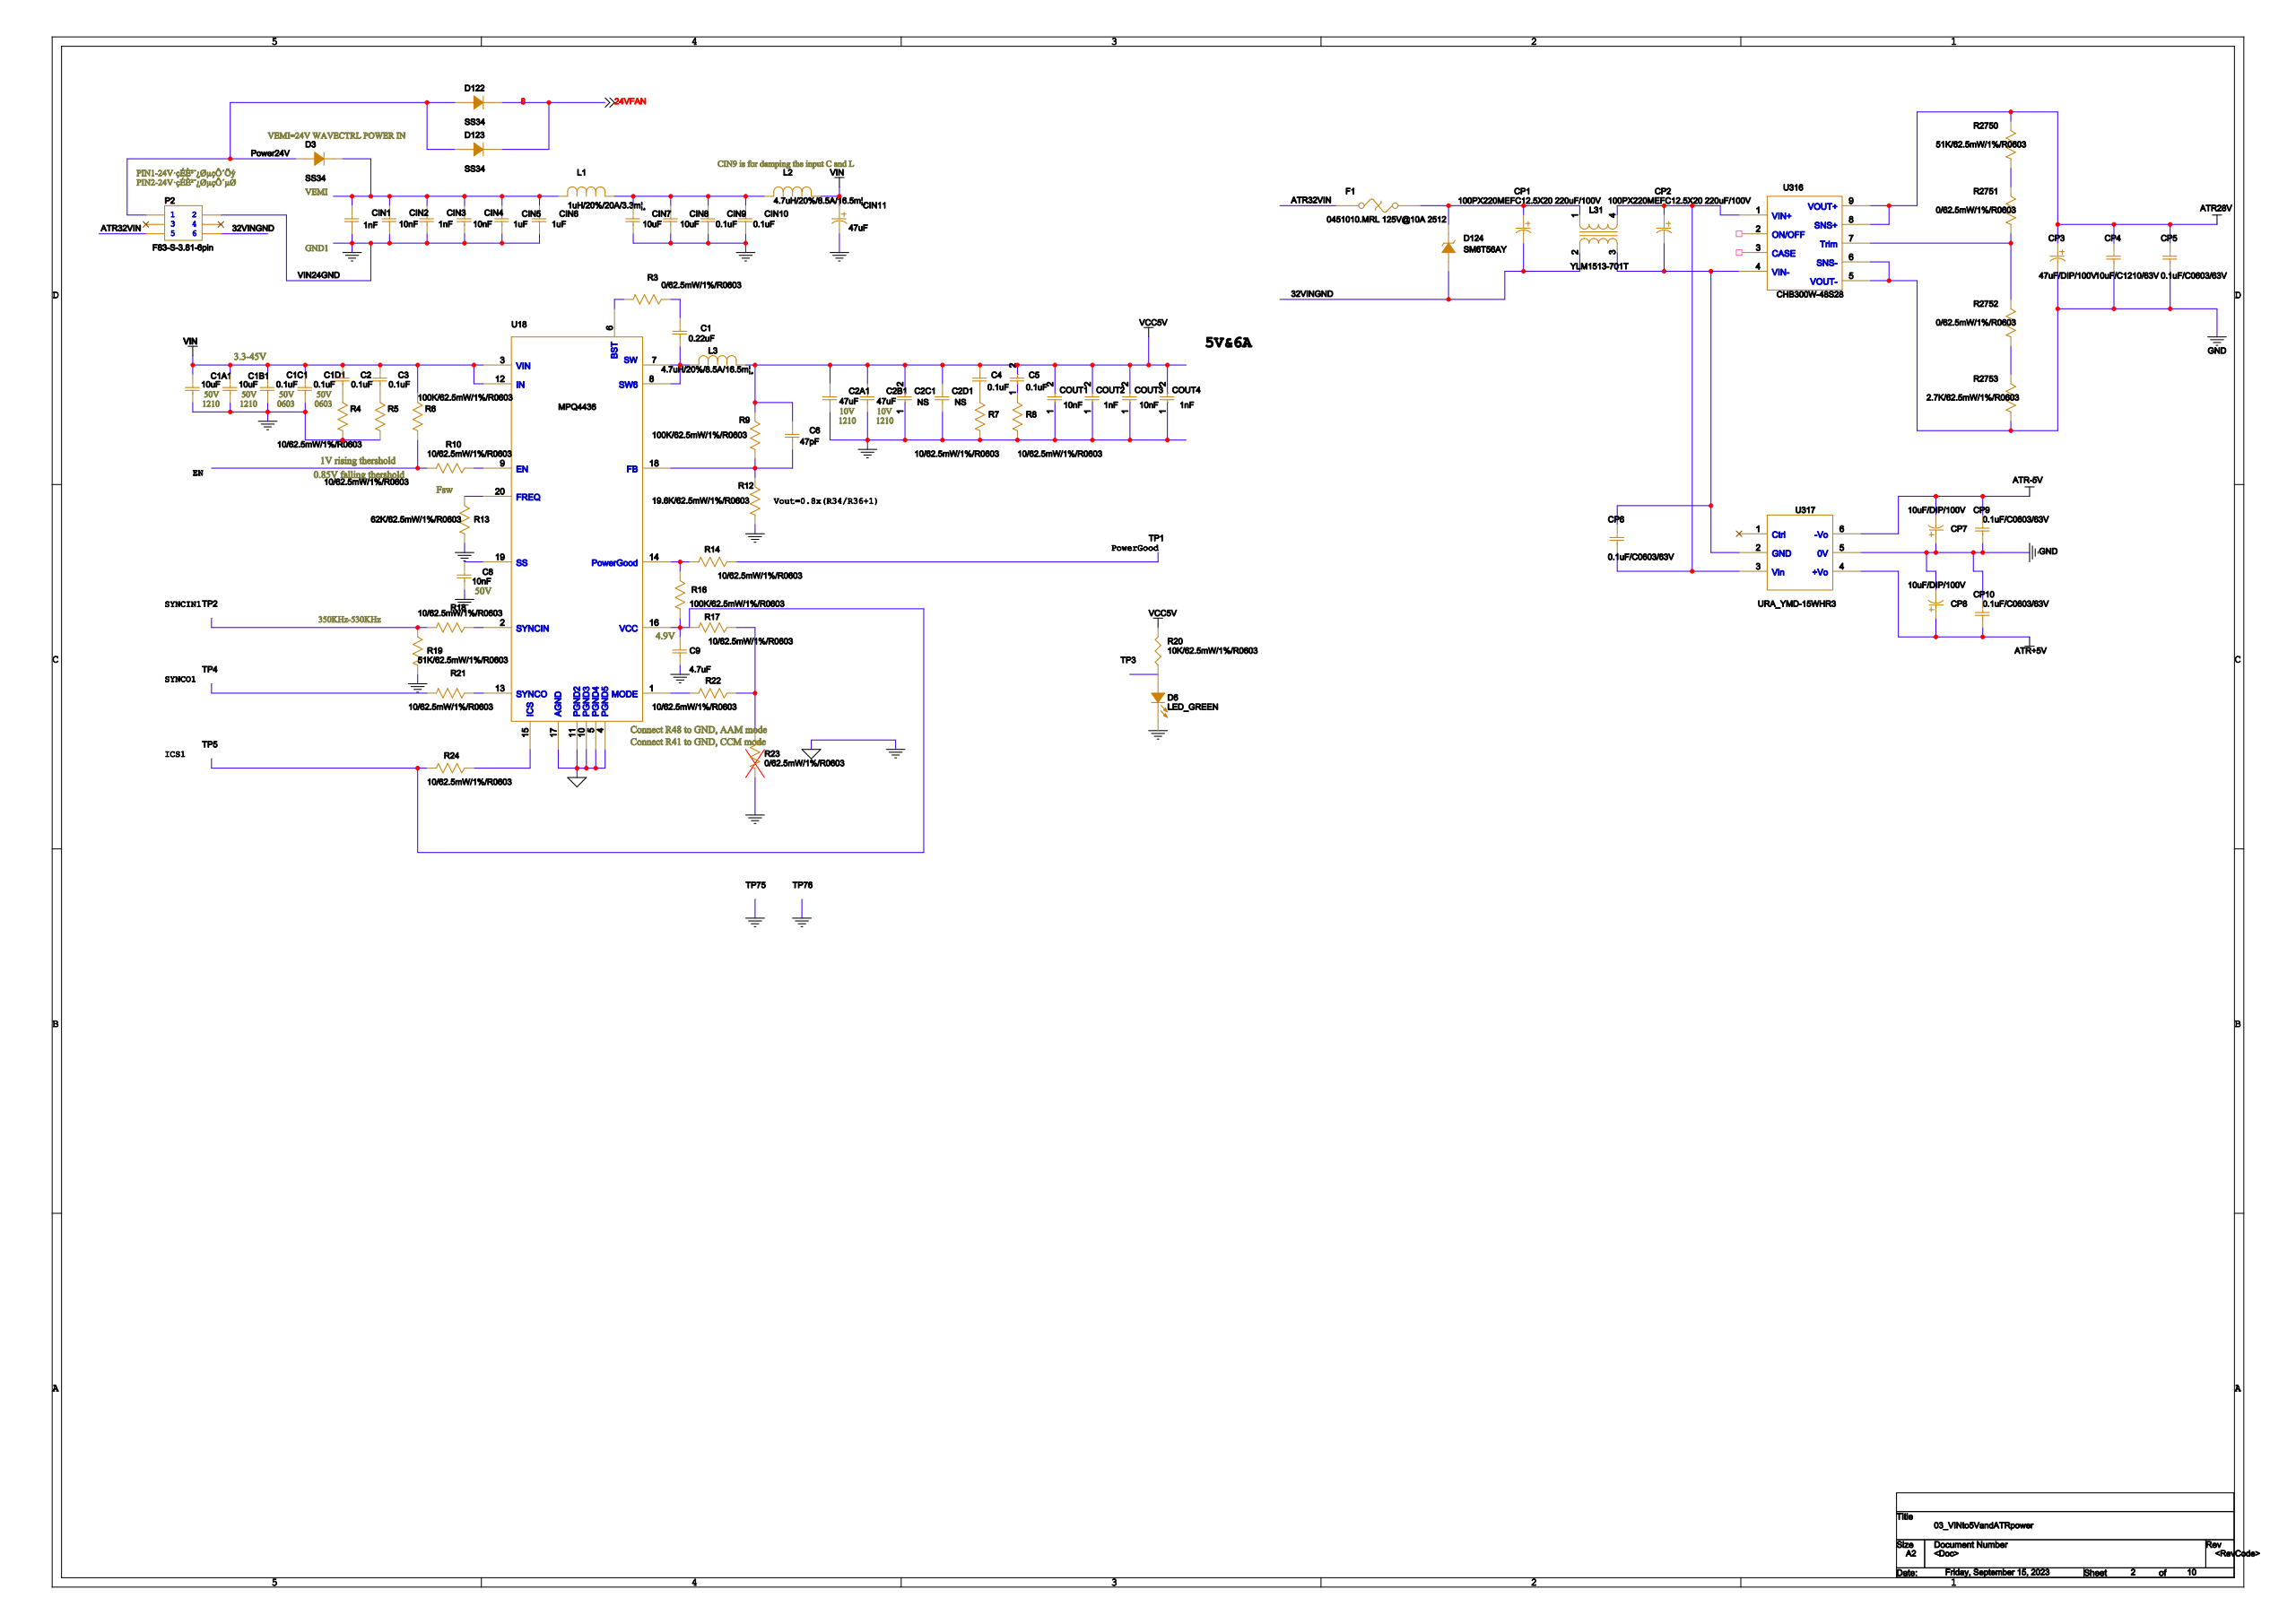Circuit board | Cadence Allegro | 634 parts | 645 nets | one sheet of the schematic
Parts on this sheet (reference | value | footprint):
C1 | CAP/0603 | 0603C
C1A1 | CAP/1210 | 1210
C1B1 | CAP/1210 | 1210
C1C1 | CAP/0603 | 0603C
C1D1 | CAP/0603 | 0603C
C2 | CAP/0603 | 0603C
C2A1 | CAP/1210 | 1210
C2B1 | CAP/1210 | 1210
C2C1 | CAP/0603 | 0603C
C2D1 | CAP/0603 | 0603C
C3 | CAP/0603 | 0603C
C4 | CAP/0603 | 0603C
C5 | CAP/0603 | 0603C
C6 | CAP/0603 | 0603C
C8 | CAP/0603 | 0603C
C9 | CAP/0603 | 0603C
CIN1 | CAP/0603 | 0603C
CIN2 | CAP/0603 | 0603C
CIN3 | CAP/0603 | 0603C
CIN4 | CAP/0603 | 0603C
CIN5 | CAP/0603 | 0805C
CIN6 | CAP/0603 | 0805C
CIN7 | CAP/0603 | 1206
CIN8 | CAP/0603 | 1206
CIN9 | CAP/0603 | 0603C
CIN10 | CAP/0603 | 0603C
CIN11 | CAP/ELECT/DIP/OD5.3P2.0 | AP-SMD_BD6_3-L6_6-W6_6-LS7_21
COUT1 | CAP/0603 | 0603C
COUT2 | CAP/0603 | 0603C
COUT3 | CAP/0603 | 0603C
COUT4 | CAP/0603 | 0603C
CP1 | CAP/ELECT/DIP/OD5.3P2.0 | AP-SMD_BD12_5-L20
CP2 | CAP/ELECT/DIP/OD5.3P2.0 | AP-SMD_BD12_5-L20
CP3 | CAP/ELECT/DIP/OD5.3P2.0 | AP-SMD_BD6_3-L6_6-W6_6-LS7_21
CP4 | CAP/1210 | 1210
CP5 | CAP/0603 | 0603C
CP6 | CAP/0603 | 0603C
CP7 | CAP/ELECT/DIP/OD5.3P2.0 | AP-SMD_BD6_3-L6_6-W6_6-LS7_21
CP8 | CAP/ELECT/DIP/OD5.3P2.0 | AP-SMD_BD6_3-L6_6-W6_6-LS7_21
CP9 | CAP/0603 | 0603C
CP10 | CAP/0603 | 0603C
D3 | SS34 | DO-214AC
D6 | LED_GREEN | LED0805
D122 | SS34 | DO-214AC
D123 | SS34 | DO-214AC
D124 | SM6T56AY | DO-214AA
F1 | 0451010.MRL 125V@10A 2512 | 2512
L1 | CKST1004-1uH/M-B | SMD_10X11
L2 | CKST1004-4.7uH/M | SMD_10X11
L3 | CKST1004-4.7uH/M | SMD_10X11
L31 | YLM1513-701T | SMD_7X6MM
P2 | F83-S-3.81-6pin | F83-S-3_81-6PIN
R3 | 0/62.5mW/1%/R0603 | 0603R
R4 | 10/62.5mW/1%/R0603 | 0603R
R5 | 10/62.5mW/1%/R0603 | 0603R
R6 | 100K/62.5mW/1%/R0603 | 0603R
R7 | 10/62.5mW/1%/R0603 | 0603R
R8 | 10/62.5mW/1%/R0603 | 0603R
R9 | 100K/62.5mW/1%/R0603 | 0603R
R10 | 10/62.5mW/1%/R0603 | 0603R
R12 | 19.6K/62.5mW/1%/R0603 | 0603R
R13 | 62K/62.5mW/1%/R0603 | 0603R
R14 | 10/62.5mW/1%/R0603 | 0603R
R16 | 100K/62.5mW/1%/R0603 | 0603R
R17 | 10/62.5mW/1%/R0603 | 0603R
R18 | 10/62.5mW/1%/R0603 | 0603R
R19 | 51K/62.5mW/1%/R0603 | 0603R
R20 | 10K/62.5mW/1%/R0603 | 0603R
R21 | 10/62.5mW/1%/R0603 | 0603R
R22 | 10/62.5mW/1%/R0603 | 0603R
R23 | 0/62.5mW/1%/R0603 | 0603R
R24 | 10/62.5mW/1%/R0603 | 0603R
R2751 | 0/62.5mW/1%/R0603 | 0603R
R2752 | 0/62.5mW/1%/R0603 | 0603R
R2753 | 2.7K/62.5mW/1%/R0603 | 0603R
TP1 | TEST POINT A | TEST_12MM
TP2 | TEST POINT A | TEST_12MM
TP3 | TEST POINT A | TEST_12MM
TP4 | TEST POINT A | TEST_12MM
TP5 | TEST POINT A | TEST_12MM
TP75 | TEST POINT A | TEST_1MM
TP76 | TEST POINT A | TEST_1MM
U18 | MPQ4436 | QFN-4X4_MPQ4436-AEC1_MNP
U316 | CHB300W-48S28 | CHB300W-48S28
U317 | URA_YMD-15WHR3 | URA_YMD-15WHR3
Nets of these parts (net: part-pin ...):
ATR+5V: CP8-1 CP10-2 U317-4
AGND: C1A1-2 C1B1-2 C1C1-2 C1D1-2 C2A1-2 C2B1-2 C2C1-1 C2D1-1 C8-2 C9-2 CIN1-2 CIN2-2 CIN3-2 CIN4-2 CIN5-2 CIN6-2 CIN7-2 CIN8-2 CIN9-2 CIN10-2 CIN11-2 COUT1-1 COUT2-1 COUT3-1 COUT4-1 CP3-2 CP4-2 CP5-2 CP7-1 CP8-2 CP9-2 CP10-1 D6-2 P2-2 R4-2 R5-2 R7-2 R8-2 R12-1 R13-2 R19-1 R23-2 R2753-1 TP75-1 TP76-1 U18-4 U18-5 U18-10 U18-11 U18-17 U316-5 U316-6 U317-5
ATR28V: CP3-1 CP4-1 CP5-1 U316-8 U316-9
N24674723: CP1-1 D124-1 F1-2 L31-1
32VINGND: CP1-2 D124-2 L31-2 P2-6
N24674699: CP2-1 CP6-2 L31-4 U316-1 U317-3
N24674686: CP2-2 CP6-1 L31-3 U316-4 U317-2
ATR32VIN: F1-1 P2-5
POWER24V: D3-1 D122-1 D123-1 P2-1
N24674860: R2751-2
N24674863: R2751-1 R2752-2 U316-7
N24674857: R2752-1 R2753-2
ATR-5V: CP7-2 CP9-1 U317-6
VCC5V: C2A1-1 C2B1-1 C2C1-2 C2D1-2 C4-2 C5-2 C6-1 COUT1-2 COUT2-2 COUT3-2 COUT4-2 L3-2 R9-2 R20-2
24VFAN: D122-2 D123-2
N24666131: CIN1-1 CIN2-1 CIN3-1 CIN4-1 CIN5-1 CIN6-1 D3-2 L1-1
N24666754: C1-1 R3-2
N24666231: C1-2 L3-1 U18-7 U18-8
N24666744: R6-1 R10-1
N24666742: R10-2 U18-9
N24666764: C6-2 R9-1 R12-2 U18-18
N24666668: R13-1 U18-20
N24666078: R14-1 TP1-1
N24666732: R14-2 R16-2 U18-14
N24666090: C9-1 R16-1 R17-2 R24-2 TP5-1 U18-16
N24666113: R17-1 R22-1 R23-1
N24666054: R18-1 R19-2 TP2-1
N24666670: R18-2 U18-2
N24666066: R21-1 TP4-1
N24666720: R21-2 U18-13
N24666730: R22-2 U18-1
N24666724: R24-1 U18-15
N24666750: R3-1 U18-6
VIN: C1A1-1 C1B1-1 C1C1-1 C1D1-1 C2-1 C3-1 CIN11-1 L2-2 R6-2 U18-3 U18-12
N24666666: C8-1 U18-19
N246663090: C4-1 R7-1
N246662770: C2-2 R4-1
N246664821: C3-2 R5-1
N24666921: C5-1 R8-1
N24666698: CIN7-1 CIN8-1 CIN9-1 CIN10-1 L1-2 L2-1
N24666963: D6-1 R20-1 TP3-1